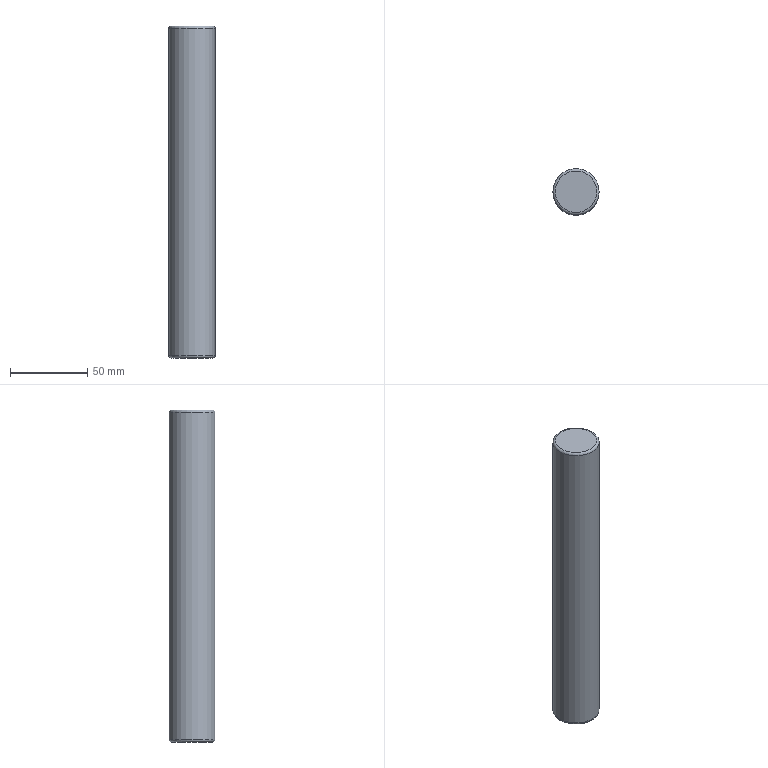Part | STEP file | solid 59 | 1 solid | 5 faces | box 30 x 30 x 215.5 mm | volume 152239 mm3 | plane 2 | torus 2 | cylinder 1 | commonest cylinder face diameters 30 x1